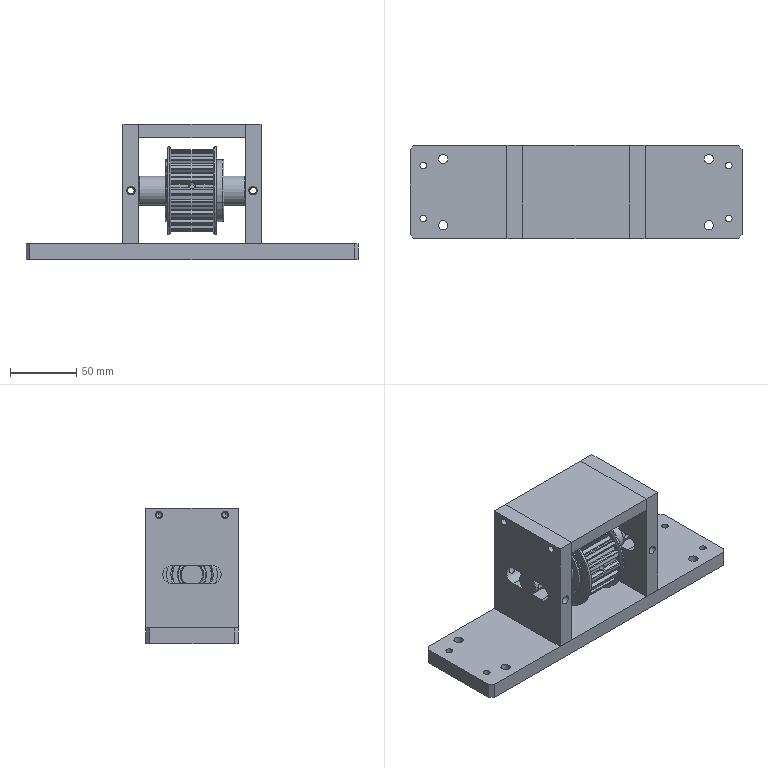Part | SolidWorks | features AEMSimFeature 1 | 12 solids | 621 faces | box 250 x 70 x 102 mm | volume 529348 mm3 | cylinder 263 | plane 142 | torus 106 | sphere 56 | cone 50 | spline 4 | commonest cylinder face diameters 1 x50 1.2 x50 55.4 x23 5 x20 61.8 x20 7 x16